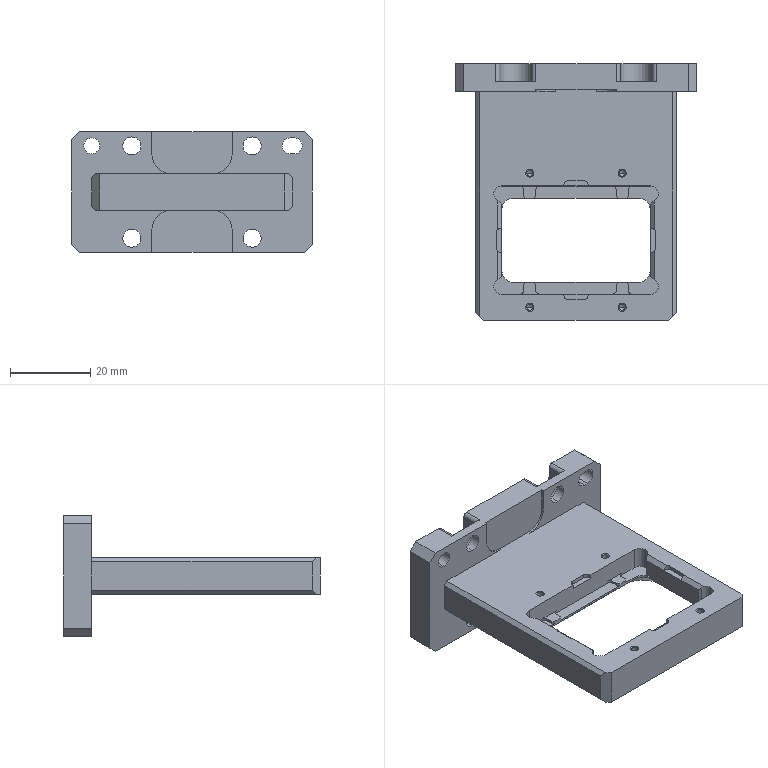NC program | NX | posted with a generic post | part box 60 x 64 x 30 mm
Lines 1 to 31 of 12381:
N10 G17 G21 G94 G90
(FLOOR_WALL , TOOL : D20R0.8)
N12 T01 M6
N14 G54
N16 G17 G0 G90 X47. Y-31.999 B0. C0. S7500 M3
N18 G43 Z30. H1
N20 Z3.
N22 G94 G1 Z0. F1350.
N24 X44.
N26 X-44.
N28 Y-27.659
N30 Y-22.559
N32 X44.
N34 Y-13.119
N36 X-44.
N38 Y-3.68
N40 X44.
N42 Y5.76
N44 X-44.
N46 Y15.2
N48 X44.
N50 Y24.64
N52 X-44.
N54 X-47.
N56 Z3.
N58 G0 Z30.
N60 M5